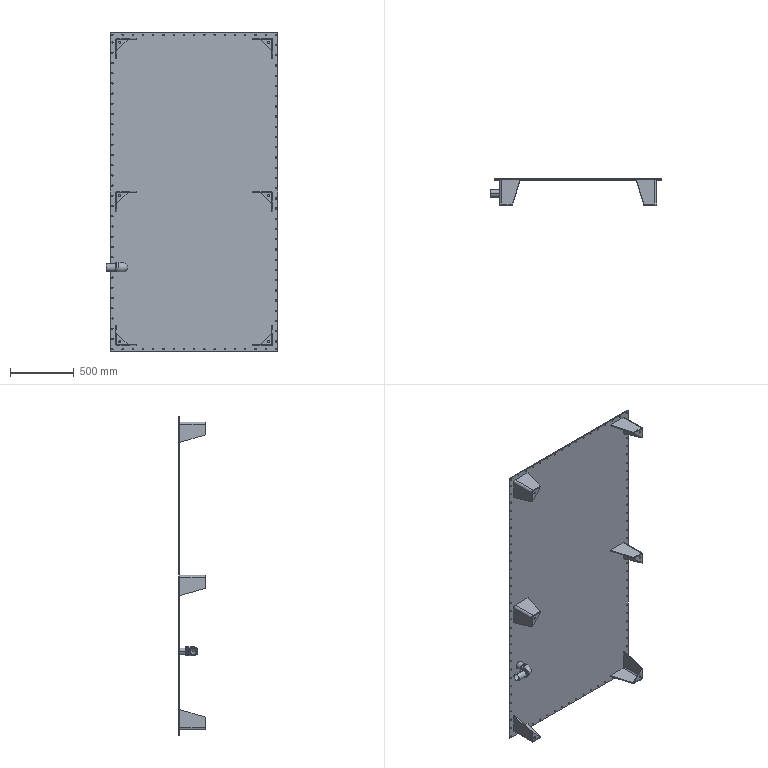Part | SolidWorks | features CompositeCurve 1 | 16 solids | 371 faces | box 1344 x 208 x 2490 mm | volume 28773491 mm3 | cylinder 234 | plane 120 | torus 11 | cone 6 | commonest cylinder face diameters 10 x188 16 x12 60 x8 20 x6 36 x6 53 x4